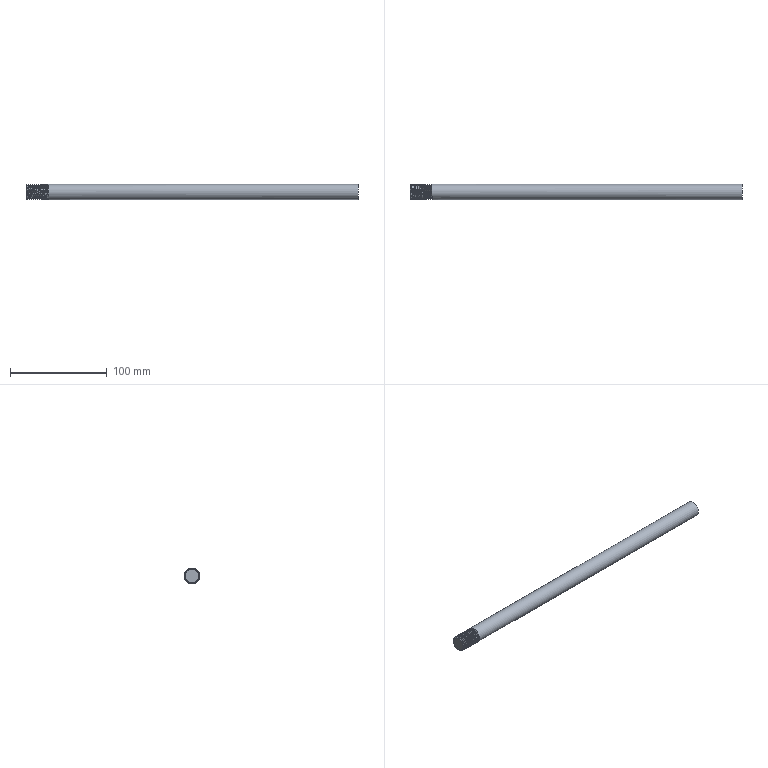Part | STEP file | Tube feed_id794_x_t | 1 solid | 19 faces | box 344 x 16 x 16 mm | volume 68432 mm3 | cylinder 13 | plane 3 | spline 2 | cone 1 | commonest cylinder face diameters 16 x12 14 x1